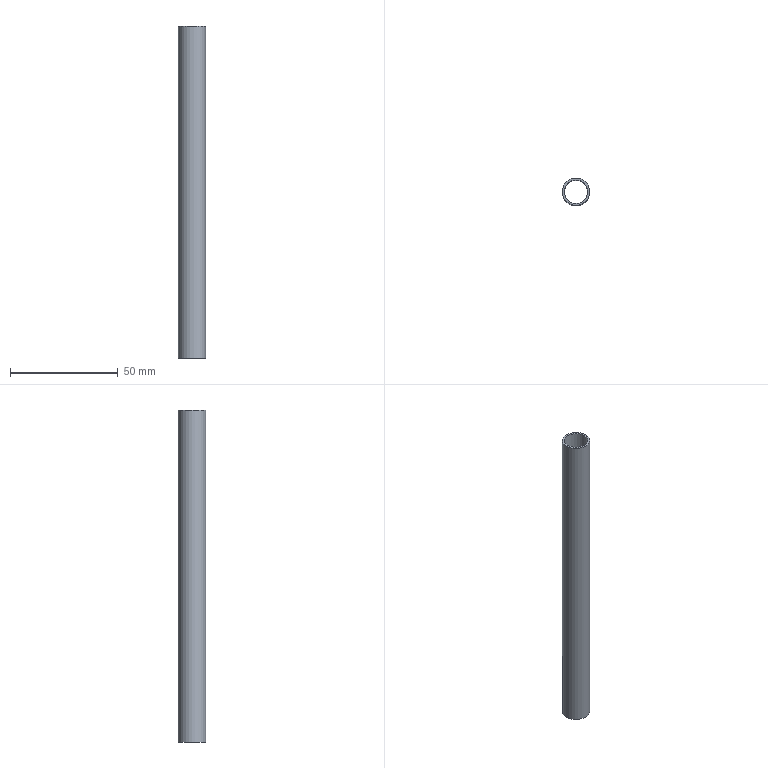Part | NX | features solid 2 | 1 solid | 4 faces | box 12.7 x 12.7 x 154 mm | volume 5080 mm3 | cylinder 2 | plane 2 | commonest cylinder face diameters 10.922 x1 12.7 x1
STEP:
#1=CARTESIAN_POINT('',(6.35,0.,154.));
#2=VERTEX_POINT('',#1);
#3=CARTESIAN_POINT('',(0.,0.,154.));
#4=DIRECTION('',(0.,0.,1.));
#5=DIRECTION('',(1.,0.,0.));
#6=AXIS2_PLACEMENT_3D('',#3,#4,#5);
#7=CIRCLE('',#6,6.35);
#8=EDGE_CURVE('',#2,#2,#7,.T.);
#9=ORIENTED_EDGE('',*,*,#8,.F.);
#10=EDGE_LOOP('',(#9));
#11=FACE_BOUND('',#10,.T.);
#12=CARTESIAN_POINT('',(6.35,0.,0.));
#13=VERTEX_POINT('',#12);
#14=CARTESIAN_POINT('',(0.,0.,0.));
#15=DIRECTION('',(0.,0.,1.));
#16=DIRECTION('',(1.,0.,0.));
#17=AXIS2_PLACEMENT_3D('',#14,#15,#16);
#18=CIRCLE('',#17,6.35);
#19=EDGE_CURVE('',#13,#13,#18,.T.);
#20=ORIENTED_EDGE('',*,*,#19,.T.);
#21=EDGE_LOOP('',(#20));
#22=FACE_BOUND('',#21,.T.);
#23=CARTESIAN_POINT('',(0.,0.,154.));
#24=DIRECTION('',(0.,0.,-1.));
#25=DIRECTION('',(-1.,0.,0.));
#26=AXIS2_PLACEMENT_3D('',#23,#24,#25);
#27=CYLINDRICAL_SURFACE('',#26,6.35);
#28=ADVANCED_FACE('',(#11,#22),#27,.T.);
#29=CARTESIAN_POINT('',(5.461,0.,154.));
#30=VERTEX_POINT('',#29);
#31=CARTESIAN_POINT('',(0.,0.,154.));
#32=DIRECTION('',(0.,0.,1.));
#33=DIRECTION('',(1.,0.,0.));
#34=AXIS2_PLACEMENT_3D('',#31,#32,#33);
#35=CIRCLE('',#34,5.461);
#36=EDGE_CURVE('',#30,#30,#35,.T.);
#37=ORIENTED_EDGE('',*,*,#36,.T.);
#38=EDGE_LOOP('',(#37));
#39=FACE_BOUND('',#38,.T.);
#40=CARTESIAN_POINT('',(5.461,0.,0.));
#41=VERTEX_POINT('',#40);
#42=CARTESIAN_POINT('',(0.,0.,0.));
#43=DIRECTION('',(0.,0.,1.));
#44=DIRECTION('',(1.,0.,0.));
#45=AXIS2_PLACEMENT_3D('',#42,#43,#44);
#46=CIRCLE('',#45,5.461);
#47=EDGE_CURVE('',#41,#41,#46,.T.);
#48=ORIENTED_EDGE('',*,*,#47,.F.);
#49=EDGE_LOOP('',(#48));
#50=FACE_BOUND('',#49,.T.);
#51=CARTESIAN_POINT('',(0.,0.,154.));
#52=DIRECTION('',(0.,0.,-1.));
#53=DIRECTION('',(-1.,0.,0.));
#54=AXIS2_PLACEMENT_3D('',#51,#52,#53);
#55=CYLINDRICAL_SURFACE('',#54,5.461);
#56=ADVANCED_FACE('',(#39,#50),#55,.F.);
#57=ORIENTED_EDGE('',*,*,#8,.T.);
#58=EDGE_LOOP('',(#57));
#59=FACE_BOUND('',#58,.T.);
#60=ORIENTED_EDGE('',*,*,#36,.F.);
#61=EDGE_LOOP('',(#60));
#62=FACE_BOUND('',#61,.T.);
#63=CARTESIAN_POINT('',(0.,0.,154.));
#64=DIRECTION('',(0.,0.,1.));
#65=DIRECTION('',(1.,0.,0.));
#66=AXIS2_PLACEMENT_3D('',#63,#64,#65);
#67=PLANE('',#66);
#68=ADVANCED_FACE('',(#59,#62),#67,.T.);
#69=ORIENTED_EDGE('',*,*,#19,.F.);
#70=EDGE_LOOP('',(#69));
#71=FACE_BOUND('',#70,.T.);
#72=ORIENTED_EDGE('',*,*,#47,.T.);
#73=EDGE_LOOP('',(#72));
#74=FACE_BOUND('',#73,.T.);
#75=CARTESIAN_POINT('',(0.,0.,0.));
#76=DIRECTION('',(0.,0.,1.));
#77=DIRECTION('',(1.,0.,0.));
#78=AXIS2_PLACEMENT_3D('',#75,#76,#77);
#79=PLANE('',#78);
#80=ADVANCED_FACE('',(#71,#74),#79,.F.);
#81=CLOSED_SHELL('',(#28,#56,#68,#80));
#82=MANIFOLD_SOLID_BREP('',#81);
#83=(LENGTH_UNIT()NAMED_UNIT(*)SI_UNIT(.MILLI.,.METRE.));
#84=UNCERTAINTY_MEASURE_WITH_UNIT(LENGTH_MEASURE(0.00001),#83,'','');
#85=(NAMED_UNIT(*)PLANE_ANGLE_UNIT()SI_UNIT($,.RADIAN.));
#86=(NAMED_UNIT(*)SI_UNIT($,.STERADIAN.)SOLID_ANGLE_UNIT());
#87=(GEOMETRIC_REPRESENTATION_CONTEXT(3)GLOBAL_UNCERTAINTY_ASSIGNED_CONTEXT((#84))GLOBAL_UNIT_ASSIGNED_CONTEXT((#83,#85,#86))REPRESENTATION_CONTEXT('',''));
#88=ADVANCED_BREP_SHAPE_REPRESENTATION('',(#82),#87);